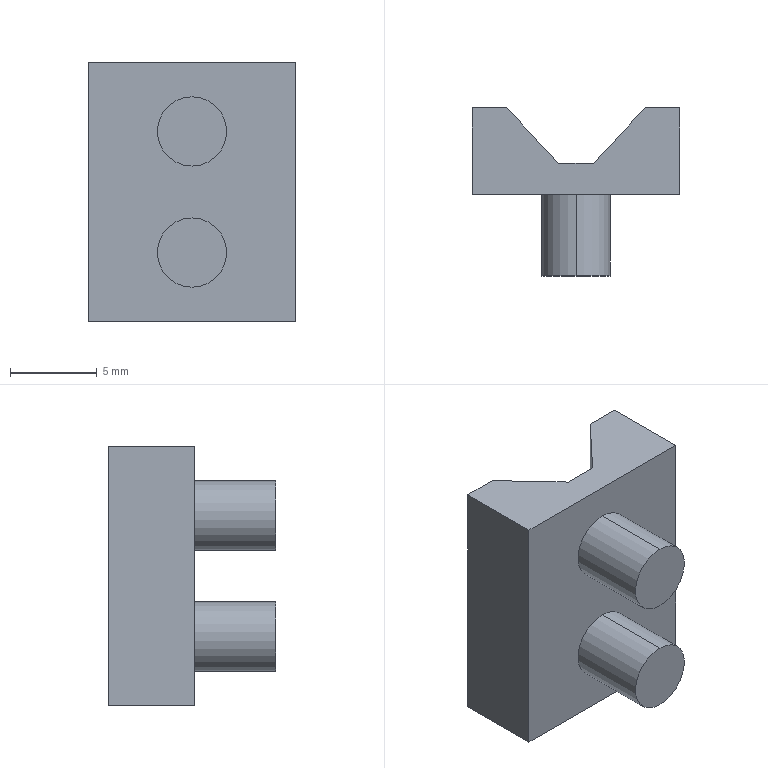Part | 1 solid | 16 faces | box 12 x 9.7 x 15 mm | volume 778.124 mm3 | plane 12 | cylinder 4 | commonest cylinder face diameters 4 x4
STEP:
#1=CARTESIAN_POINT('',(0.,-7.2,-5.5));
#2=VERTEX_POINT('',#1);
#3=CARTESIAN_POINT('',(0.,-7.2,-1.5));
#4=VERTEX_POINT('',#3);
#5=CARTESIAN_POINT('',(0.,-7.2,-3.5));
#6=DIRECTION('',(0.,-1.,0.));
#7=DIRECTION('',(0.,0.,-1.));
#8=AXIS2_PLACEMENT_3D('',#5,#6,#7);
#9=CIRCLE('',#8,2.);
#10=EDGE_CURVE('',#2,#4,#9,.T.);
#11=ORIENTED_EDGE('',*,*,#10,.F.);
#12=CARTESIAN_POINT('',(0.,-2.5,-5.5));
#13=VERTEX_POINT('',#12);
#14=CARTESIAN_POINT('',(0.,-7.2,-5.5));
#15=DIRECTION('',(0.,1.,0.));
#16=VECTOR('',#15,1000.);
#17=LINE('',#14,#16);
#18=EDGE_CURVE('',#2,#13,#17,.T.);
#19=ORIENTED_EDGE('',*,*,#18,.T.);
#20=CARTESIAN_POINT('',(0.,-2.5,-1.5));
#21=VERTEX_POINT('',#20);
#22=CARTESIAN_POINT('',(0.,-2.5,-3.5));
#23=DIRECTION('',(0.,-1.,0.));
#24=DIRECTION('',(0.,0.,1.));
#25=AXIS2_PLACEMENT_3D('',#22,#23,#24);
#26=CIRCLE('',#25,2.);
#27=EDGE_CURVE('',#13,#21,#26,.T.);
#28=ORIENTED_EDGE('',*,*,#27,.T.);
#29=CARTESIAN_POINT('',(0.,-7.2,-1.5));
#30=DIRECTION('',(0.,1.,0.));
#31=VECTOR('',#30,1000.);
#32=LINE('',#29,#31);
#33=EDGE_CURVE('',#4,#21,#32,.T.);
#34=ORIENTED_EDGE('',*,*,#33,.F.);
#35=EDGE_LOOP('',(#11,#19,#28,#34));
#36=FACE_OUTER_BOUND('',#35,.T.);
#37=CARTESIAN_POINT('',(0.,-7.2,-3.5));
#38=DIRECTION('',(0.,1.,0.));
#39=DIRECTION('',(0.,0.,1.));
#40=AXIS2_PLACEMENT_3D('',#37,#38,#39);
#41=CYLINDRICAL_SURFACE('',#40,2.);
#42=ADVANCED_FACE('',(#36),#41,.T.);
#43=CARTESIAN_POINT('',(0.,-7.2,1.5));
#44=VERTEX_POINT('',#43);
#45=CARTESIAN_POINT('',(0.,-7.2,5.5));
#46=VERTEX_POINT('',#45);
#47=CARTESIAN_POINT('',(0.,-7.2,3.5));
#48=DIRECTION('',(0.,-1.,0.));
#49=DIRECTION('',(0.,0.,-1.));
#50=AXIS2_PLACEMENT_3D('',#47,#48,#49);
#51=CIRCLE('',#50,2.);
#52=EDGE_CURVE('',#44,#46,#51,.T.);
#53=ORIENTED_EDGE('',*,*,#52,.F.);
#54=CARTESIAN_POINT('',(0.,-2.5,1.5));
#55=VERTEX_POINT('',#54);
#56=CARTESIAN_POINT('',(0.,-7.2,1.5));
#57=DIRECTION('',(0.,1.,0.));
#58=VECTOR('',#57,1000.);
#59=LINE('',#56,#58);
#60=EDGE_CURVE('',#44,#55,#59,.T.);
#61=ORIENTED_EDGE('',*,*,#60,.T.);
#62=CARTESIAN_POINT('',(0.,-2.5,5.5));
#63=VERTEX_POINT('',#62);
#64=CARTESIAN_POINT('',(0.,-2.5,3.5));
#65=DIRECTION('',(0.,-1.,0.));
#66=DIRECTION('',(0.,0.,1.));
#67=AXIS2_PLACEMENT_3D('',#64,#65,#66);
#68=CIRCLE('',#67,2.);
#69=EDGE_CURVE('',#55,#63,#68,.T.);
#70=ORIENTED_EDGE('',*,*,#69,.T.);
#71=CARTESIAN_POINT('',(0.,-7.2,5.5));
#72=DIRECTION('',(0.,1.,0.));
#73=VECTOR('',#72,1000.);
#74=LINE('',#71,#73);
#75=EDGE_CURVE('',#46,#63,#74,.T.);
#76=ORIENTED_EDGE('',*,*,#75,.F.);
#77=EDGE_LOOP('',(#53,#61,#70,#76));
#78=FACE_OUTER_BOUND('',#77,.T.);
#79=CARTESIAN_POINT('',(0.,-7.2,3.5));
#80=DIRECTION('',(0.,1.,0.));
#81=DIRECTION('',(0.,0.,1.));
#82=AXIS2_PLACEMENT_3D('',#79,#80,#81);
#83=CYLINDRICAL_SURFACE('',#82,2.);
#84=ADVANCED_FACE('',(#78),#83,.T.);
#85=CARTESIAN_POINT('',(0.,-2.5,3.5));
#86=DIRECTION('',(0.,-1.,0.));
#87=DIRECTION('',(0.,0.,1.));
#88=AXIS2_PLACEMENT_3D('',#85,#86,#87);
#89=CIRCLE('',#88,2.);
#90=EDGE_CURVE('',#63,#55,#89,.T.);
#91=ORIENTED_EDGE('',*,*,#90,.F.);
#92=ORIENTED_EDGE('',*,*,#69,.F.);
#93=EDGE_LOOP('',(#91,#92));
#94=FACE_BOUND('',#93,.T.);
#95=CARTESIAN_POINT('',(-6.,-2.5,-7.5));
#96=VERTEX_POINT('',#95);
#97=CARTESIAN_POINT('',(6.,-2.5,-7.5));
#98=VERTEX_POINT('',#97);
#99=CARTESIAN_POINT('',(-6.,-2.5,-7.5));
#100=DIRECTION('',(1.,0.,0.));
#101=VECTOR('',#100,1000.);
#102=LINE('',#99,#101);
#103=EDGE_CURVE('',#96,#98,#102,.T.);
#104=ORIENTED_EDGE('',*,*,#103,.T.);
#105=CARTESIAN_POINT('',(6.,-2.5,7.5));
#106=VERTEX_POINT('',#105);
#107=CARTESIAN_POINT('',(6.,-2.5,7.5));
#108=DIRECTION('',(0.,0.,-1.));
#109=VECTOR('',#108,1000.);
#110=LINE('',#107,#109);
#111=EDGE_CURVE('',#106,#98,#110,.T.);
#112=ORIENTED_EDGE('',*,*,#111,.F.);
#113=CARTESIAN_POINT('',(-6.,-2.5,7.5));
#114=VERTEX_POINT('',#113);
#115=CARTESIAN_POINT('',(-6.,-2.5,7.5));
#116=DIRECTION('',(1.,0.,0.));
#117=VECTOR('',#116,1000.);
#118=LINE('',#115,#117);
#119=EDGE_CURVE('',#114,#106,#118,.T.);
#120=ORIENTED_EDGE('',*,*,#119,.F.);
#121=CARTESIAN_POINT('',(-6.,-2.5,7.5));
#122=DIRECTION('',(0.,0.,-1.));
#123=VECTOR('',#122,1000.);
#124=LINE('',#121,#123);
#125=EDGE_CURVE('',#114,#96,#124,.T.);
#126=ORIENTED_EDGE('',*,*,#125,.T.);
#127=EDGE_LOOP('',(#104,#112,#120,#126));
#128=FACE_OUTER_BOUND('',#127,.T.);
#129=CARTESIAN_POINT('',(0.,-2.5,-3.5));
#130=DIRECTION('',(0.,-1.,0.));
#131=DIRECTION('',(0.,0.,1.));
#132=AXIS2_PLACEMENT_3D('',#129,#130,#131);
#133=CIRCLE('',#132,2.);
#134=EDGE_CURVE('',#21,#13,#133,.T.);
#135=ORIENTED_EDGE('',*,*,#134,.F.);
#136=ORIENTED_EDGE('',*,*,#27,.F.);
#137=EDGE_LOOP('',(#135,#136));
#138=FACE_BOUND('',#137,.T.);
#139=CARTESIAN_POINT('',(-6.,-2.5,7.5));
#140=DIRECTION('',(0.,1.,0.));
#141=DIRECTION('',(0.,0.,1.));
#142=AXIS2_PLACEMENT_3D('',#139,#140,#141);
#143=PLANE('',#142);
#144=ADVANCED_FACE('',(#94,#128,#138),#143,.F.);
#145=CARTESIAN_POINT('',(6.,2.5,-7.5));
#146=VERTEX_POINT('',#145);
#147=CARTESIAN_POINT('',(4.,2.5,-7.5));
#148=VERTEX_POINT('',#147);
#149=CARTESIAN_POINT('',(4.,2.5,-7.5));
#150=DIRECTION('',(-1.,0.,0.));
#151=VECTOR('',#150,1000.);
#152=LINE('',#149,#151);
#153=EDGE_CURVE('',#146,#148,#152,.T.);
#154=ORIENTED_EDGE('',*,*,#153,.T.);
#155=CARTESIAN_POINT('',(4.,2.5,7.5));
#156=VERTEX_POINT('',#155);
#157=CARTESIAN_POINT('',(4.,2.5,7.5));
#158=DIRECTION('',(0.,0.,-1.));
#159=VECTOR('',#158,1000.);
#160=LINE('',#157,#159);
#161=EDGE_CURVE('',#156,#148,#160,.T.);
#162=ORIENTED_EDGE('',*,*,#161,.F.);
#163=CARTESIAN_POINT('',(6.,2.5,7.5));
#164=VERTEX_POINT('',#163);
#165=CARTESIAN_POINT('',(4.,2.5,7.5));
#166=DIRECTION('',(-1.,0.,0.));
#167=VECTOR('',#166,1000.);
#168=LINE('',#165,#167);
#169=EDGE_CURVE('',#164,#156,#168,.T.);
#170=ORIENTED_EDGE('',*,*,#169,.F.);
#171=CARTESIAN_POINT('',(6.,2.5,7.5));
#172=DIRECTION('',(0.,0.,-1.));
#173=VECTOR('',#172,1000.);
#174=LINE('',#171,#173);
#175=EDGE_CURVE('',#164,#146,#174,.T.);
#176=ORIENTED_EDGE('',*,*,#175,.T.);
#177=EDGE_LOOP('',(#154,#162,#170,#176));
#178=FACE_OUTER_BOUND('',#177,.T.);
#179=CARTESIAN_POINT('',(4.,2.5,7.5));
#180=DIRECTION('',(0.,-1.,0.));
#181=DIRECTION('',(1.,0.,0.));
#182=AXIS2_PLACEMENT_3D('',#179,#180,#181);
#183=PLANE('',#182);
#184=ADVANCED_FACE('',(#178),#183,.F.);
#185=CARTESIAN_POINT('',(1.,-0.7,-7.5));
#186=VERTEX_POINT('',#185);
#187=CARTESIAN_POINT('',(4.,2.5,-7.5));
#188=DIRECTION('',(-0.6839,-0.7295,0.));
#189=VECTOR('',#188,1000.);
#190=LINE('',#187,#189);
#191=EDGE_CURVE('',#148,#186,#190,.T.);
#192=ORIENTED_EDGE('',*,*,#191,.T.);
#193=CARTESIAN_POINT('',(1.,-0.7,7.5));
#194=VERTEX_POINT('',#193);
#195=CARTESIAN_POINT('',(1.,-0.7,7.5));
#196=DIRECTION('',(0.,0.,-1.));
#197=VECTOR('',#196,1000.);
#198=LINE('',#195,#197);
#199=EDGE_CURVE('',#194,#186,#198,.T.);
#200=ORIENTED_EDGE('',*,*,#199,.F.);
#201=CARTESIAN_POINT('',(4.,2.5,7.5));
#202=DIRECTION('',(-0.6839,-0.7295,0.));
#203=VECTOR('',#202,1000.);
#204=LINE('',#201,#203);
#205=EDGE_CURVE('',#156,#194,#204,.T.);
#206=ORIENTED_EDGE('',*,*,#205,.F.);
#207=ORIENTED_EDGE('',*,*,#161,.T.);
#208=EDGE_LOOP('',(#192,#200,#206,#207));
#209=FACE_OUTER_BOUND('',#208,.T.);
#210=CARTESIAN_POINT('',(4.,2.5,7.5));
#211=DIRECTION('',(0.7295,-0.6839,0.));
#212=DIRECTION('',(0.6839,0.7295,0.));
#213=AXIS2_PLACEMENT_3D('',#210,#211,#212);
#214=PLANE('',#213);
#215=ADVANCED_FACE('',(#209),#214,.F.);
#216=CARTESIAN_POINT('',(-1.,-0.7,-7.5));
#217=VERTEX_POINT('',#216);
#218=CARTESIAN_POINT('',(-1.,-0.7,-7.5));
#219=DIRECTION('',(-1.,0.,0.));
#220=VECTOR('',#219,1000.);
#221=LINE('',#218,#220);
#222=EDGE_CURVE('',#186,#217,#221,.T.);
#223=ORIENTED_EDGE('',*,*,#222,.T.);
#224=CARTESIAN_POINT('',(-1.,-0.7,7.5));
#225=VERTEX_POINT('',#224);
#226=CARTESIAN_POINT('',(-1.,-0.7,7.5));
#227=DIRECTION('',(0.,0.,-1.));
#228=VECTOR('',#227,1000.);
#229=LINE('',#226,#228);
#230=EDGE_CURVE('',#225,#217,#229,.T.);
#231=ORIENTED_EDGE('',*,*,#230,.F.);
#232=CARTESIAN_POINT('',(-1.,-0.7,7.5));
#233=DIRECTION('',(-1.,0.,0.));
#234=VECTOR('',#233,1000.);
#235=LINE('',#232,#234);
#236=EDGE_CURVE('',#194,#225,#235,.T.);
#237=ORIENTED_EDGE('',*,*,#236,.F.);
#238=ORIENTED_EDGE('',*,*,#199,.T.);
#239=EDGE_LOOP('',(#223,#231,#237,#238));
#240=FACE_OUTER_BOUND('',#239,.T.);
#241=CARTESIAN_POINT('',(-1.,-0.7,7.5));
#242=DIRECTION('',(0.,-1.,0.));
#243=DIRECTION('',(0.,0.,-1.));
#244=AXIS2_PLACEMENT_3D('',#241,#242,#243);
#245=PLANE('',#244);
#246=ADVANCED_FACE('',(#240),#245,.F.);
#247=CARTESIAN_POINT('',(-4.,2.5,-7.5));
#248=VERTEX_POINT('',#247);
#249=CARTESIAN_POINT('',(-4.,2.5,-7.5));
#250=DIRECTION('',(-0.6839,0.7295,0.));
#251=VECTOR('',#250,1000.);
#252=LINE('',#249,#251);
#253=EDGE_CURVE('',#217,#248,#252,.T.);
#254=ORIENTED_EDGE('',*,*,#253,.T.);
#255=CARTESIAN_POINT('',(-4.,2.5,7.5));
#256=VERTEX_POINT('',#255);
#257=CARTESIAN_POINT('',(-4.,2.5,7.5));
#258=DIRECTION('',(0.,0.,-1.));
#259=VECTOR('',#258,1000.);
#260=LINE('',#257,#259);
#261=EDGE_CURVE('',#256,#248,#260,.T.);
#262=ORIENTED_EDGE('',*,*,#261,.F.);
#263=CARTESIAN_POINT('',(-4.,2.5,7.5));
#264=DIRECTION('',(-0.6839,0.7295,0.));
#265=VECTOR('',#264,1000.);
#266=LINE('',#263,#265);
#267=EDGE_CURVE('',#225,#256,#266,.T.);
#268=ORIENTED_EDGE('',*,*,#267,.F.);
#269=ORIENTED_EDGE('',*,*,#230,.T.);
#270=EDGE_LOOP('',(#254,#262,#268,#269));
#271=FACE_OUTER_BOUND('',#270,.T.);
#272=CARTESIAN_POINT('',(-4.,2.5,7.5));
#273=DIRECTION('',(-0.7295,-0.6839,0.));
#274=DIRECTION('',(0.6839,-0.7295,0.));
#275=AXIS2_PLACEMENT_3D('',#272,#273,#274);
#276=PLANE('',#275);
#277=ADVANCED_FACE('',(#271),#276,.F.);
#278=CARTESIAN_POINT('',(-6.,2.5,-7.5));
#279=VERTEX_POINT('',#278);
#280=CARTESIAN_POINT('',(-6.,2.5,-7.5));
#281=DIRECTION('',(-1.,0.,0.));
#282=VECTOR('',#281,1000.);
#283=LINE('',#280,#282);
#284=EDGE_CURVE('',#248,#279,#283,.T.);
#285=ORIENTED_EDGE('',*,*,#284,.T.);
#286=CARTESIAN_POINT('',(-6.,2.5,7.5));
#287=VERTEX_POINT('',#286);
#288=CARTESIAN_POINT('',(-6.,2.5,7.5));
#289=DIRECTION('',(0.,0.,-1.));
#290=VECTOR('',#289,1000.);
#291=LINE('',#288,#290);
#292=EDGE_CURVE('',#287,#279,#291,.T.);
#293=ORIENTED_EDGE('',*,*,#292,.F.);
#294=CARTESIAN_POINT('',(-6.,2.5,7.5));
#295=DIRECTION('',(-1.,0.,0.));
#296=VECTOR('',#295,1000.);
#297=LINE('',#294,#296);
#298=EDGE_CURVE('',#256,#287,#297,.T.);
#299=ORIENTED_EDGE('',*,*,#298,.F.);
#300=ORIENTED_EDGE('',*,*,#261,.T.);
#301=EDGE_LOOP('',(#285,#293,#299,#300));
#302=FACE_OUTER_BOUND('',#301,.T.);
#303=CARTESIAN_POINT('',(-6.,2.5,7.5));
#304=DIRECTION('',(0.,-1.,0.));
#305=DIRECTION('',(0.,0.,-1.));
#306=AXIS2_PLACEMENT_3D('',#303,#304,#305);
#307=PLANE('',#306);
#308=ADVANCED_FACE('',(#302),#307,.F.);
#309=CARTESIAN_POINT('',(-6.,-2.5,-7.5));
#310=DIRECTION('',(0.,-1.,0.));
#311=VECTOR('',#310,1000.);
#312=LINE('',#309,#311);
#313=EDGE_CURVE('',#279,#96,#312,.T.);
#314=ORIENTED_EDGE('',*,*,#313,.T.);
#315=ORIENTED_EDGE('',*,*,#125,.F.);
#316=CARTESIAN_POINT('',(-6.,-2.5,7.5));
#317=DIRECTION('',(0.,-1.,0.));
#318=VECTOR('',#317,1000.);
#319=LINE('',#316,#318);
#320=EDGE_CURVE('',#287,#114,#319,.T.);
#321=ORIENTED_EDGE('',*,*,#320,.F.);
#322=ORIENTED_EDGE('',*,*,#292,.T.);
#323=EDGE_LOOP('',(#314,#315,#321,#322));
#324=FACE_OUTER_BOUND('',#323,.T.);
#325=CARTESIAN_POINT('',(-6.,-2.5,7.5));
#326=DIRECTION('',(1.,0.,0.));
#327=DIRECTION('',(0.,0.,-1.));
#328=AXIS2_PLACEMENT_3D('',#325,#326,#327);
#329=PLANE('',#328);
#330=ADVANCED_FACE('',(#324),#329,.F.);
#331=CARTESIAN_POINT('',(6.,-2.5,-7.5));
#332=DIRECTION('',(0.,1.,0.));
#333=VECTOR('',#332,1000.);
#334=LINE('',#331,#333);
#335=EDGE_CURVE('',#98,#146,#334,.T.);
#336=ORIENTED_EDGE('',*,*,#335,.T.);
#337=ORIENTED_EDGE('',*,*,#175,.F.);
#338=CARTESIAN_POINT('',(6.,-2.5,7.5));
#339=DIRECTION('',(0.,1.,0.));
#340=VECTOR('',#339,1000.);
#341=LINE('',#338,#340);
#342=EDGE_CURVE('',#106,#164,#341,.T.);
#343=ORIENTED_EDGE('',*,*,#342,.F.);
#344=ORIENTED_EDGE('',*,*,#111,.T.);
#345=EDGE_LOOP('',(#336,#337,#343,#344));
#346=FACE_OUTER_BOUND('',#345,.T.);
#347=CARTESIAN_POINT('',(6.,-2.5,7.5));
#348=DIRECTION('',(-1.,0.,0.));
#349=DIRECTION('',(0.,0.,1.));
#350=AXIS2_PLACEMENT_3D('',#347,#348,#349);
#351=PLANE('',#350);
#352=ADVANCED_FACE('',(#346),#351,.F.);
#353=ORIENTED_EDGE('',*,*,#169,.T.);
#354=ORIENTED_EDGE('',*,*,#205,.T.);
#355=ORIENTED_EDGE('',*,*,#236,.T.);
#356=ORIENTED_EDGE('',*,*,#267,.T.);
#357=ORIENTED_EDGE('',*,*,#298,.T.);
#358=ORIENTED_EDGE('',*,*,#320,.T.);
#359=ORIENTED_EDGE('',*,*,#119,.T.);
#360=ORIENTED_EDGE('',*,*,#342,.T.);
#361=EDGE_LOOP('',(#353,#354,#355,#356,#357,#358,#359,#360));
#362=FACE_OUTER_BOUND('',#361,.T.);
#363=CARTESIAN_POINT('',(0.,0.,7.5));
#364=DIRECTION('',(0.,0.,1.));
#365=DIRECTION('',(1.,0.,0.));
#366=AXIS2_PLACEMENT_3D('',#363,#364,#365);
#367=PLANE('',#366);
#368=ADVANCED_FACE('',(#362),#367,.T.);
#369=ORIENTED_EDGE('',*,*,#153,.F.);
#370=ORIENTED_EDGE('',*,*,#335,.F.);
#371=ORIENTED_EDGE('',*,*,#103,.F.);
#372=ORIENTED_EDGE('',*,*,#313,.F.);
#373=ORIENTED_EDGE('',*,*,#284,.F.);
#374=ORIENTED_EDGE('',*,*,#253,.F.);
#375=ORIENTED_EDGE('',*,*,#222,.F.);
#376=ORIENTED_EDGE('',*,*,#191,.F.);
#377=EDGE_LOOP('',(#369,#370,#371,#372,#373,#374,#375,#376));
#378=FACE_OUTER_BOUND('',#377,.T.);
#379=CARTESIAN_POINT('',(0.,0.,-7.5));
#380=DIRECTION('',(0.,0.,1.));
#381=DIRECTION('',(1.,0.,0.));
#382=AXIS2_PLACEMENT_3D('',#379,#380,#381);
#383=PLANE('',#382);
#384=ADVANCED_FACE('',(#378),#383,.F.);
#385=ORIENTED_EDGE('',*,*,#60,.F.);
#386=CARTESIAN_POINT('',(0.,-7.2,3.5));
#387=DIRECTION('',(0.,-1.,0.));
#388=DIRECTION('',(0.,0.,-1.));
#389=AXIS2_PLACEMENT_3D('',#386,#387,#388);
#390=CIRCLE('',#389,2.);
#391=EDGE_CURVE('',#46,#44,#390,.T.);
#392=ORIENTED_EDGE('',*,*,#391,.F.);
#393=ORIENTED_EDGE('',*,*,#75,.T.);
#394=ORIENTED_EDGE('',*,*,#90,.T.);
#395=EDGE_LOOP('',(#385,#392,#393,#394));
#396=FACE_OUTER_BOUND('',#395,.T.);
#397=CARTESIAN_POINT('',(0.,-7.2,3.5));
#398=DIRECTION('',(0.,1.,0.));
#399=DIRECTION('',(0.,0.,1.));
#400=AXIS2_PLACEMENT_3D('',#397,#398,#399);
#401=CYLINDRICAL_SURFACE('',#400,2.);
#402=ADVANCED_FACE('',(#396),#401,.T.);
#403=ORIENTED_EDGE('',*,*,#391,.T.);
#404=ORIENTED_EDGE('',*,*,#52,.T.);
#405=EDGE_LOOP('',(#403,#404));
#406=FACE_OUTER_BOUND('',#405,.T.);
#407=CARTESIAN_POINT('',(0.,-7.2,3.5));
#408=DIRECTION('',(0.,-1.,0.));
#409=DIRECTION('',(0.,0.,-1.));
#410=AXIS2_PLACEMENT_3D('',#407,#408,#409);
#411=PLANE('',#410);
#412=ADVANCED_FACE('',(#406),#411,.T.);
#413=ORIENTED_EDGE('',*,*,#18,.F.);
#414=CARTESIAN_POINT('',(0.,-7.2,-3.5));
#415=DIRECTION('',(0.,-1.,0.));
#416=DIRECTION('',(0.,0.,-1.));
#417=AXIS2_PLACEMENT_3D('',#414,#415,#416);
#418=CIRCLE('',#417,2.);
#419=EDGE_CURVE('',#4,#2,#418,.T.);
#420=ORIENTED_EDGE('',*,*,#419,.F.);
#421=ORIENTED_EDGE('',*,*,#33,.T.);
#422=ORIENTED_EDGE('',*,*,#134,.T.);
#423=EDGE_LOOP('',(#413,#420,#421,#422));
#424=FACE_OUTER_BOUND('',#423,.T.);
#425=CARTESIAN_POINT('',(0.,-7.2,-3.5));
#426=DIRECTION('',(0.,1.,0.));
#427=DIRECTION('',(0.,0.,1.));
#428=AXIS2_PLACEMENT_3D('',#425,#426,#427);
#429=CYLINDRICAL_SURFACE('',#428,2.);
#430=ADVANCED_FACE('',(#424),#429,.T.);
#431=ORIENTED_EDGE('',*,*,#419,.T.);
#432=ORIENTED_EDGE('',*,*,#10,.T.);
#433=EDGE_LOOP('',(#431,#432));
#434=FACE_OUTER_BOUND('',#433,.T.);
#435=CARTESIAN_POINT('',(0.,-7.2,-3.5));
#436=DIRECTION('',(0.,-1.,0.));
#437=DIRECTION('',(0.,0.,-1.));
#438=AXIS2_PLACEMENT_3D('',#435,#436,#437);
#439=PLANE('',#438);
#440=ADVANCED_FACE('',(#434),#439,.T.);
#441=CLOSED_SHELL('',(#42,#84,#144,#184,#215,#246,#277,#308,#330,#352,#368,#384,#402,#412,#430,#440));
#442=MANIFOLD_SOLID_BREP('',#441);
#443=CARTESIAN_POINT('',(0.,0.,0.));
#444=DIRECTION('',(0.,0.,1.));
#445=DIRECTION('',(1.,0.,0.));
#446=AXIS2_PLACEMENT_3D('',#443,#444,#445);
#447=(LENGTH_UNIT()NAMED_UNIT(*)SI_UNIT(.MILLI.,.METRE.));
#448=UNCERTAINTY_MEASURE_WITH_UNIT(LENGTH_MEASURE(0.00001),#447,'','');
#449=(NAMED_UNIT(*)PLANE_ANGLE_UNIT()SI_UNIT($,.RADIAN.));
#450=(NAMED_UNIT(*)SI_UNIT($,.STERADIAN.)SOLID_ANGLE_UNIT());
#451=(GEOMETRIC_REPRESENTATION_CONTEXT(3)GLOBAL_UNCERTAINTY_ASSIGNED_CONTEXT((#448))GLOBAL_UNIT_ASSIGNED_CONTEXT((#447,#449,#450))REPRESENTATION_CONTEXT('',''));
#452=ADVANCED_BREP_SHAPE_REPRESENTATION('',(#442,#446),#451);